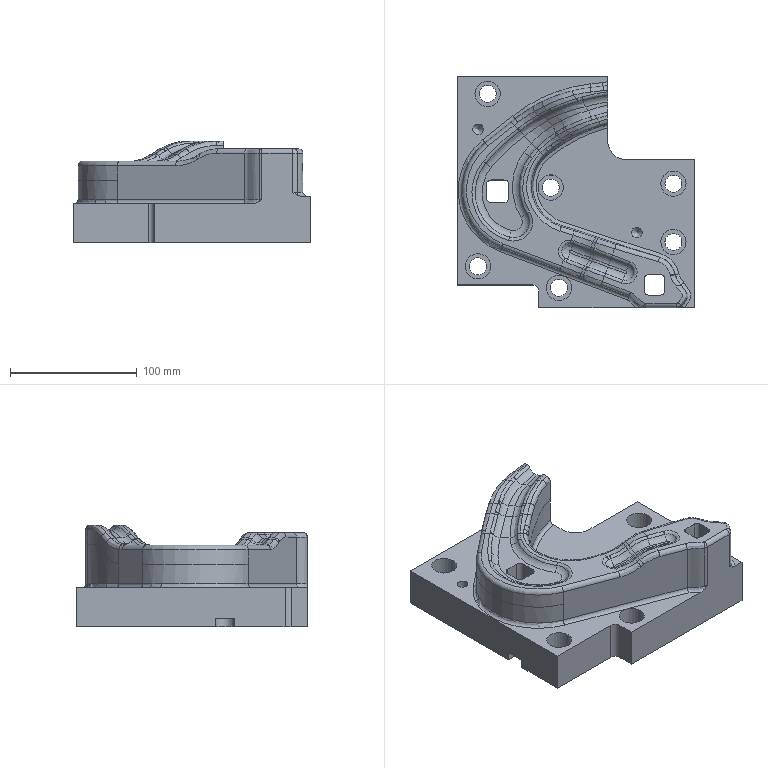Part | NX | features 23 2 | 1 solid | 232 faces | box 188 x 183 x 80.4 mm | volume 1264073 mm3 | cylinder 71 | spline 71 | plane 58 | torus 30 | cone 2 | commonest cylinder face diameters 6 x11 7 x7 10 x7 13.5 x6 20 x6 8 x4